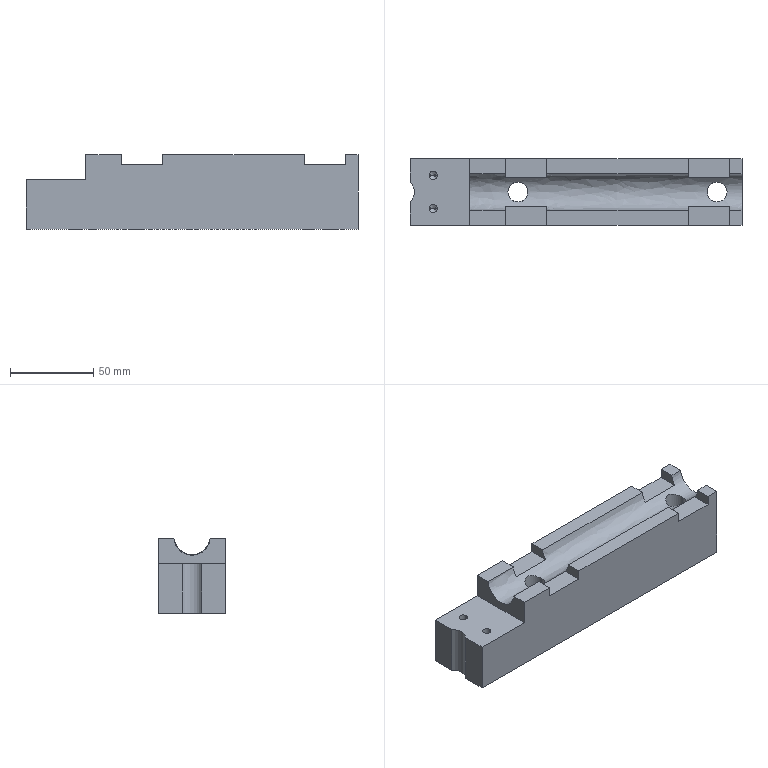NC program | NX | posted with a generic post
Lines 51 to 871 of 104568:
(ADAPTIVE_MILLING , TOOL : D10)
N100 T10 M6
N102 G54
N104 G17 G0 G90 X-107.551 Y-7.025 S9500 M3
N106 G43 Z30. H10
N108 Z-14.
N110 G94 G1 Z-15. F1000.
N112 X-105.318 Y-5.203 F3000.
N114 G3 X-104.997 Y-4.734 R1.064
N116 X-104.349 Y-0.599 R14.499
N118 X-104.258 Y2.898 R266.437
N120 X-104.741 Y3.891 R4.524
N122 G1 X-104.988 Y4.652
N124 G3 X-106.825 Y5.076 R1.102
N126 X-107.131 Y4.103 Z-14.947 R1.226
N128 G1 X-107.114 Y3.158 Z-14.9
N130 X-107.007 Y-2.847
N132 X-107. Y-3.483 Z-14.932
N134 X-106.969 Y-4.118 Z-14.964
N136 G3 X-106.617 Y-4.74 Z-15. R1.142
N138 X-104.842 Y-4.258 R1.102
N140 G2 X-104.254 Y-2.857 R24.923
N142 G3 X-103.658 Y2.081 R14.394
N144 X-104.235 Y2.995 R2.49
N146 G1 X-104.386 Y3.255
N148 G3 X-106.437 Y2.738 R1.101
N150 G1 X-106.619 Y-3.004
N152 G3 X-104.568 Y-3.591 R1.101
N154 X-103.136 Y1.38 R8.223
N156 X-103.8 Y2.451 R1.628
N158 G1 X-103.863 Y2.529
N160 G3 X-105.812 Y1.902 R1.101
N162 G1 X-106.065 Y-2.065
N164 G3 X-104.124 Y-2.842 R1.101
N166 X-102.749 Y1.145 R4.895
N168 G1 X-102.781 Y1.24
N170 X-102.821 Y1.331
N172 X-102.869 Y1.419
N174 G3 X-104.769 Y1.098 R1.102
N176 G1 X-105.607 Y-1.299
N178 G3 X-103.764 Y-2.412 R1.1
N180 X-102.442 Y-0.209 R3.842
N182 X-103.406 Y2.063 R2.803
N184 X-105.271 Y1.184 R1.101
N186 G1 X-105.076 Y-1.145
N188 G3 X-103.126 Y-1.747 R1.101
N190 X-102.442 Y-0.159 R2.495
N192 X-103.99 Y0.696 R1.012
N194 G1 X-104.991 Y0.067
N196 Z-12.
N198 G0 Z30.
N200 X-71.498 Y-27.794
N202 Z-13.849
N204 G1 Z-14.849 F1000.
N206 X-69.324 Y-25.783 F3000.
N208 G3 X-69. Y-25.042 R1.036
N210 X-71.916 Y-24.421 R8.181
N212 X-81.712 Y-24.21 R140.093
N214 G1 X-84.812 Y-24.207
N216 X-93.112 Y-24.205
N218 X-97.212
N220 X-97.312
N222 X-97.412 Y-24.203
N224 X-97.512 Y-24.198
N226 X-97.611 Y-24.192
N228 X-97.711 Y-24.183
N230 G2 X-102.043 Y-21.266 R6.063
N232 X-103.851 Y-15.497 R13.384
N234 X-104.115 Y-7.608 R54.303
N236 X-102.845 Y-3.623 R13.92
N238 G3 X-101.964 Y-0.266 R8.163
N240 X-102.667 Y1.898 R4.856
N242 G2 X-103.964 Y7.723 R17.087
N244 X-104.151 Y17.818 R129.978
N246 X-101.162 Y22.103 R6.099
N248 X-95.574 Y23.842 R13.466
N250 X-86.185 Y24.177 R90.73
N252 G3 X-70.586 Y24.227 R873.779
N254 X-69.295 Y24.665 R1.839
N256 X-69.022 Y25.112 R0.67
N258 X-69.69 Y26.058 R1.016
N260 G1 X-71.526 Y26.85 Z-14.749
N262 X-72.651 Y27.325
N264 X-72.919 Y27.362
N266 X-91.044
N268 G3 X-97.219 Y26.684 R28.808
N270 G1 X-98.437 Y26.413
N272 X-99.643 Y26.097
N274 G3 X-102.893 Y24.694 R14.612
N276 X-104.94 Y23.028 R10.254
N278 X-106.011 Y21.74 R8.094
N280 X-106.589 Y20.468 R5.588
N282 X-107.179 Y17.218 R15.413
N284 G1 X-107.231 Y16.391
N286 X-107.264 Y15.563
N288 X-107.597 Y-2.565
N290 G3 X-107.069 Y-13.778 R86.922
N292 G1 X-106.855 Y-15.681
N294 X-106.627 Y-17.583
N296 G3 X-105.191 Y-21.981 R14.894
N298 X-103.057 Y-24.999 R11.047
N300 G1 X-102.589 Y-25.467
N302 X-102.086 Y-25.898
N304 G3 X-100.53 Y-26.655 R4.838
N306 X-97.263 Y-27.212 R18.153
N308 G1 X-95.606 Y-27.319
N310 X-72.182 Y-28.224
N312 G3 X-71.516 Y-28.003 R1.032
N314 G1 X-70.11 Y-26.581 Z-14.849
N316 X-69.641 Y-26.109
N318 X-69.187 Y-25.623
N320 G3 X-69. Y-25.042 R1.045
N322 X-71.055 Y-24.079 R4.12
N324 X-77.516 Y-23.485 R33.131
N326 X-94.916 Y-23.403 R929.638
N328 G2 X-101.065 Y-19.485 R7.672
N330 X-102.98 Y-13.22 R15.729
N332 X-102.373 Y-5.318 R17.042
N334 G3 X-101.445 Y-1.132 R17.421
N336 X-101.971 Y1.806 R9.318
N338 G2 X-103.266 Y11.496 R40.447
N340 X-103.269 Y15.592 R31.14
N342 X-99.192 Y21.213 R7.783
N344 X-92.989 Y23.004 R16.193
N346 X-82.5 Y23.368 R104.354
N348 G3 X-71.702 Y23.449 R294.043
N350 X-69.296 Y24.284 R3.808
N352 X-69.022 Y25.021 R1.24
N354 X-69.691 Y25.969 R1.017
N356 G1 X-71.526 Y26.765 Z-14.749
N358 X-72.638 Y27.236
N360 X-72.919 Y27.271
N362 X-76.041 Y27.221
N364 X-79.162 Y27.12
N366 X-80.721 Y27.027
N368 X-82.278 Y26.917
N370 X-93.991 Y25.966
N372 G3 X-100.261 Y24.168 R16.575
N374 X-103.666 Y21.525 R13.673
N376 X-105.578 Y18.422 R7.953
N378 X-106.274 Y14.774 R14.488
N380 G1 X-106.563 Y9.89
N382 X-106.828 Y5.005
N384 G3 X-106.502 Y-8.29 R101.645
N386 G1 X-106.248 Y-11.134
N388 X-105.974 Y-13.977
N390 G3 X-104.543 Y-19.27 R19.249
N392 X-102.584 Y-22.402 R14.036
N394 G1 X-101.515 Y-23.672
N396 G3 X-98.586 Y-25.633 R8.09
N398 X-95.198 Y-26.339 R10.609
N400 G1 X-72.897 Y-27.292
N402 X-72.671 Y-27.272
N404 X-72.453 Y-27.208
N406 X-71.527 Y-26.802
N408 X-69.695 Y-26. Z-14.849
N410 G3 X-69. Y-25.042 R1.028
N412 X-70.551 Y-23.847 R2.838
N414 X-75.737 Y-22.862 R17.231
N416 X-87.532 Y-22.628 R195.199
N418 G2 X-93.331 Y-22.567 R112.761
N420 X-100.282 Y-17.783 R8.839
N422 X-101.664 Y-6.706 R16.242
N424 G3 X-100.864 Y-1.978 R34.974
N426 X-101.188 Y1.298 R14.457
N428 G2 X-102.425 Y13.113 R58.709
N430 X-97.864 Y20.191 R8.624
N432 X-91.193 Y22.152 R17.537
N434 X-81.706 Y22.549 R91.712
N436 G3 X-72.708 Y22.666 R202.321
N438 X-69.585 Y23.594 R6.019
N440 X-69.022 Y25.004 R1.448
N442 X-69.546 Y25.885 R1.011
N444 X-70.167 Y26.013 Z-14.817 R1.33
N446 G1 X-71.524 Y26.08 Z-14.749
N448 X-73.368 Y26.169
N450 X-77.742 Y26.174
N452 X-82.115 Y26.156
N454 G3 X-90.8 Y25.347 R61.155
N456 G1 X-94.989 Y24.639
N458 G3 X-99.124 Y22.965 R12.448
N460 G1 X-101.144 Y21.662
N462 G3 X-104.145 Y18.28 R9.835
N464 X-104.913 Y16.113 R8.633
N466 X-105.57 Y10.565 R27.18
N468 G1 X-105.757 Y-6.313
N470 G3 X-105.168 Y-12.5 R29.708
N472 X-104.358 Y-15.897 R32.087
N474 X-101.843 Y-21.056 R18.258
N476 X-98.772 Y-23.951 R11.298
N478 X-95.759 Y-25.144 R9.712
N480 X-92.685 Y-25.546 R16.686
N482 G1 X-73.263 Y-26.206
N484 X-71.527 Y-26.119
N486 X-69.811 Y-26.024 Z-14.835
N488 X-69.547 Y-25.933 Z-14.849
N490 G3 X-69. Y-25.042 R1.011
N492 X-70.13 Y-23.706 R2.222
N494 X-74.492 Y-22.349 R11.492
N496 X-83.774 Y-21.867 R75.922
N498 G2 X-91.572 Y-21.767 R185.382
N500 X-99.539 Y-16.175 R9.697
N502 X-100.826 Y-8.385 R14.411
N504 G3 X-100.227 Y-3.019 R231.829
N506 X-100.616 Y2.157 R25.935
N508 G2 X-101.499 Y11.306 R64.597
N510 X-96.577 Y19.253 R9.266
N512 X-89.524 Y21.322 R18.611
N514 X-78.537 Y21.747 R107.245
N516 G3 X-72.448 Y22.016 R46.627
N518 X-69.433 Y23.238 R5.711
N520 X-69.022 Y24.52 R1.468
N522 X-69.547 Y25.4 R1.011
N524 X-70.167 Y25.529 Z-14.817 R1.331
N526 G1 X-71.525 Y25.595 Z-14.749
N528 X-73.369 Y25.685
N530 X-77.534 Y25.673
N532 G3 X-82.716 Y25.272 R48.529
N534 G1 X-87.362 Y24.658
N536 X-92.005 Y24.022
N538 G3 X-98.894 Y21.283 R17.826
N540 X-101.285 Y19.489 R17.961
N542 X-103.973 Y14.822 R9.419
N544 X-104.324 Y12.737 R15.756
N546 X-104.616 Y9.008 R43.847
N548 X-104.645 Y1.146 R94.064
N550 G1 X-104.565 Y-0.349
N552 X-103.778 Y-12.828
N554 G3 X-102.349 Y-17.548 R10.682
N556 G1 X-100.862 Y-20.052
N558 G3 X-99.013 Y-21.984 R8.138
N560 X-94.577 Y-24.179 R12.587
N562 X-90.918 Y-24.867 R17.239
N564 G1 X-73.347 Y-26.206
N566 X-71.525 Y-26.121
N568 X-69.809 Y-26.023 Z-14.835
N570 X-69.544 Y-25.932 Z-14.849
N572 G3 X-69. Y-25.042 R1.011
N574 X-69.875 Y-23.538 R2.003
N576 X-73.699 Y-21.895 R9.077
N578 X-81.652 Y-21.144 R44.159
N580 G2 X-89.949 Y-20.975 R319.751
N582 X-99.206 Y-13.243 R10.229
N584 X-99.672 Y-6.99 R18.982
N586 G3 X-99.991 Y3.18 R42.362
N588 G2 X-100.553 Y9.752 R61.219
N590 X-95.226 Y18.421 R9.799
N592 X-87.966 Y20.499 R19.673
N594 X-77.78 Y20.945 R110.754
N596 G3 X-72.209 Y21.411 R29.071
N598 X-69.3 Y22.861 R5.501
N600 X-69.022 Y24.108 R1.707
N602 X-69.547 Y24.988 R1.011
N604 X-70.164 Y25.117 Z-14.817 R1.336
N606 G1 X-71.525 Y25.189 Z-14.749
N608 X-73.206 Y25.277
N610 X-73.369 Y25.272
N612 X-87.154 Y23.741
N614 G3 X-94.199 Y22.172 R33.647
N616 G1 X-95.251 Y21.815
N618 X-96.284 Y21.406
N620 G3 X-99.404 Y19.237 R10.854
N622 X-101.784 Y16.276 R13.511
N624 X-103.571 Y12.698 R44.582
N626 X-103.932 Y10.637 R5.47
N628 G1 X-103.599 Y-4.359
N630 G3 X-102.683 Y-11.765 R37.364
N632 G1 X-102.353 Y-13.227
N634 X-102.003 Y-14.685
N636 G3 X-101.245 Y-16.51 R9.099
N638 X-99.657 Y-19.043 R27.673
N640 X-97.843 Y-20.922 R11.68
N642 X-93.539 Y-23.281 R11.51
N644 X-91.118 Y-23.807 R15.167
N646 G1 X-73.256 Y-26.114
N648 X-71.525 Y-26.025
N650 X-69.808 Y-25.923 Z-14.835
N652 X-69.545 Y-25.832 Z-14.849
N654 G3 X-69. Y-24.942 R1.011
N656 X-69.906 Y-23.131 R2.265
N658 X-73.848 Y-21.275 R9.175
N660 X-81.485 Y-20.404 R38.939
N662 G2 X-88.68 Y-20.17 R205.805
N664 X-98.068 Y-12.319 R10.298
N666 X-98.679 Y-6.569 R22.003
N668 G3 X-99.267 Y3.706 R76.468
N670 G2 X-99.576 Y9.191 R34.592
N672 X-94.017 Y17.553 R10.207
N674 X-86.56 Y19.67 R20.395
N676 X-77.276 Y20.161 R125.201
N678 G3 X-71.837 Y20.871 R22.237
N680 X-69.213 Y22.432 R5.181
N682 X-69.023 Y23.581 R1.938
N684 X-69.6 Y24.488 R1.011
N686 X-70.505 Y24.479 Z-14.803 R1.154
N688 G1 X-71.525 Y24.161 Z-14.749
N690 X-72.452 Y23.87
N692 X-73.383 Y23.594
N694 X-75.013 Y23.543
N696 X-76.644 Y23.515
N698 G3 X-82.871 Y23.123 R76.701
N700 G1 X-85.461 Y22.853
N702 X-88.049 Y22.562
N704 G3 X-93.852 Y21.015 R25.49
N706 X-96.659 Y19.433 R15.104
N708 X-99.778 Y16.884 R27.516
N710 X-100.947 Y15.216 R6.294
N712 X-102.075 Y12.449 R24.754
N714 X-102.429 Y10.499 R8.848
N716 G1 X-102.575 Y8.186
N718 X-102.673 Y5.869
N720 G3 X-102.495 Y0.53 R51.707
N722 G1 X-101.629 Y-9.434
N724 G3 X-100.383 Y-14.868 R20.192
N726 X-98.162 Y-18.554 R13.351
N728 G1 X-97.017 Y-19.872
N730 G3 X-93.242 Y-22.175 R8.847
N732 X-88.993 Y-23.091 R20.48
N734 G1 X-73.403 Y-24.656
N736 X-71.527 Y-25.222
N738 X-70.153 Y-25.63 Z-14.821
N740 G3 X-69.599 Y-25.558 Z-14.849 R1.055
N742 X-69. Y-24.642 R1.01
N744 X-69.979 Y-22.646 R2.559
N746 X-74.061 Y-20.625 R9.568
N748 X-82.284 Y-19.627 R39.178
N750 G2 X-88.27 Y-19.274 R57.428
N752 X-96.862 Y-11.745 R10.375
N754 X-97.763 Y-5.526 R25.703
N756 G3 X-98.637 Y5.839 R344.55
N758 G2 X-97.195 Y12.674 R11.496
N760 X-90.93 Y17.565 R12.06
N762 X-83.096 Y19.049 R28.641
N764 G3 X-75.113 Y19.554 R220.804
N766 X-70.337 Y20.908 R12.291
N768 X-69.077 Y22.148 R2.767
N770 X-69.023 Y23.012 R4.341
N772 X-69.6 Y23.919 R1.011
N774 X-70.505 Y23.91 Z-14.803 R1.155
N776 G1 X-71.526 Y23.594 Z-14.749
N778 X-73.39 Y23.025
N780 X-76.017 Y22.929
N782 G3 X-80.986 Y22.517 R51.887
N784 G1 X-86.769 Y21.735
N786 G3 X-92.168 Y20.362 R29.535
N788 X-95.372 Y18.835 R21.075
N790 G1 X-96.799 Y17.979
N792 G3 X-98.255 Y16.556 R6.064
N794 X-100.231 Y13.382 R25.609
N796 X-101.584 Y9.382 R14.544
N798 X-101.716 Y7.399 R10.601
N800 G1 X-101.567 Y2.492
N802 X-101.394 Y-2.415
N804 G3 X-100.638 Y-8.782 R50.316
N806 G1 X-100.172 Y-11.235
N808 G3 X-97.267 Y-17.365 R15.298
N810 G1 X-96.558 Y-18.26
N812 X-95.838 Y-19.145
N814 G3 X-93.807 Y-20.672 R6.888
N816 X-91.362 Y-21.581 R12.433
N818 X-87.709 Y-22.363 R26.648
N820 G1 X-73.5 Y-24.342
N822 X-73.349 Y-24.375
N824 X-71.525 Y-24.926
N826 X-70.151 Y-25.33 Z-14.821
N828 G3 X-69.596 Y-25.256 Z-14.849 R1.054
N830 X-69. Y-24.342 R1.01
N832 X-70.022 Y-22.15 R2.81
N834 X-74.245 Y-19.971 R9.919
N836 X-82.255 Y-18.884 R37.047
N838 G2 X-87.823 Y-18.355 R34.863
N840 X-95.565 Y-11.515 R10.527
N842 X-96.885 Y-4.865 R25.565
N844 X-97.736 Y5.198 R295.524
N846 X-95.266 Y13.017 R11.166
N848 X-88.537 Y17.129 R13.662
N850 X-80.544 Y18.333 R37.68
N852 G3 X-73.688 Y19.065 R53.452
N854 X-69.682 Y20.777 R9.113
N856 X-69.023 Y22.422 R1.695
N858 X-69.599 Y23.328 R1.011
N860 X-70.5 Y23.323 Z-14.803 R1.157
N862 G1 X-71.526 Y23.012 Z-14.749
N864 X-73.357 Y22.457
N866 X-73.523 Y22.422
N868 X-84.686 Y21.027
N870 G3 X-91.319 Y19.355 R28.821
N872 X-94.793 Y17.433 R18.207
N874 X-97.379 Y15.413 R29.622
N876 X-99.15 Y12.943 R8.08
N878 X-99.893 Y10.958 R14.071
N880 X-100.635 Y7.311 R17.458
N882 X-100.819 Y1.284 R50.62
N884 X-100.502 Y-2.025 R31.857
N886 G1 X-99.946 Y-5.732
N888 X-99.367 Y-9.435
N890 G3 X-96.735 Y-15.692 R16.082
N892 X-95.247 Y-17.693 R25.842
N894 X-94.334 Y-18.535 R5.886
N896 X-91.25 Y-20.406 R15.587
N898 X-89.356 Y-21.004 R10.183
N900 X-79.553 Y-22.939 R395.254
N902 G1 X-73.392 Y-24.068
N904 X-71.522 Y-24.629
N906 X-70.149 Y-25.03 Z-14.821
N908 G3 X-69.593 Y-24.955 Z-14.849 R1.054
N910 X-69. Y-24.042 R1.01
N912 X-70.043 Y-21.65 R3.006
N914 X-74.406 Y-19.311 R10.29
N916 X-81.804 Y-18.169 R35.029
N918 G2 X-87.245 Y-17.442 R27.777
N920 X-94.402 Y-10.969 R10.885
N922 X-96.066 Y-3.886 R26.04
N924 X-96.815 Y4.677 R87.751
N926 X-90.536 Y15.039 R11.199
N928 X-82.975 Y17.181 R22.418
N930 G3 X-75.325 Y18.043 R321.614
N932 X-70.324 Y19.687 R13.269
N934 X-69.079 Y20.948 R2.96
N936 G1 X-69.052 Y21.044
N938 X-69.033 Y21.142
N940 G3 X-69.546 Y22.131 R1.01
N942 X-70.197 Y22.258 Z-14.816 R1.286
N944 G1 X-71.525 Y22.283 Z-14.749
N946 X-73.219 Y22.316
N948 X-73.379 Y22.307
N950 X-78.326 Y21.587
N952 G3 X-84.424 Y20.266 R62.869
N954 G1 X-86.644 Y19.667
N956 X-88.86 Y19.051
N958 G3 X-94.826 Y15.787 R17.967
N960 X-96.851 Y13.767 R19.041
N962 X-98.751 Y10.293 R10.937
N964 X-99.764 Y2.334 R18.501
N966 G1 X-99.441 Y-1.222
N968 X-99.096 Y-4.776
N970 G3 X-97.986 Y-9.99 R30.679
N972 G1 X-97.652 Y-11.076
N974 X-97.273 Y-12.146
N976 G3 X-95.956 Y-14.603 R13.344
N978 X-93.96 Y-17.113 R15.83
N980 X-91.994 Y-18.622 R9.756
N982 X-88.001 Y-20.293 R13.57
N984 G1 X-73.439 Y-23.658
N986 X-71.527 Y-24.229
N988 X-70.149 Y-24.63 Z-14.821
N990 G3 X-69.597 Y-24.557 Z-14.849 R1.055
N992 X-69. Y-23.642 R1.01
N994 X-70.048 Y-21.144 R3.159
N996 X-74.359 Y-18.708 R10.402
N998 X-81.733 Y-17.425 R35.048
N1000 G2 X-87.295 Y-16.281 R19.663
N1002 X-93.571 Y-9.756 R11.657
N1004 X-95.303 Y-2.686 R28.378
N1006 X-95.856 Y4.383 R42.163
N1008 X-89.464 Y14.191 R11.366
N1010 X-82.01 Y16.358 R23.26
N1012 G3 X-74.688 Y17.419 R130.567
N1014 X-69.985 Y19.29 R12.043
N1016 X-69.127 Y20.415 R1.86
N1018 X-69.024 Y21.919 R8.71
N1020 X-69.598 Y22.824 R1.011
N1022 X-70.497 Y22.822 Z-14.803 R1.158
N1024 G1 X-71.527 Y22.514 Z-14.749
N1026 X-73.524 Y21.919
N1028 X-84.438 Y19.19
N1030 G3 X-90.893 Y16.895 R35.793
N1032 X-94.35 Y14.689 R18.634
N1034 X-96.158 Y12.643 R11.095
N1036 X-97.987 Y9.39 R20.489
N1038 X-99.025 Y5.554 R13.162
N1040 X-99.051 Y3.338 R14.817
N1042 X-98.545 Y-1.626 R40.301
N1044 G1 X-98.097 Y-4.337
N1046 X-97.626 Y-7.044
N1048 G3 X-95.463 Y-12.943 R21.269
N1050 X-92.778 Y-16.327 R14.939
N1052 X-89.082 Y-18.774 R11.611
N1054 X-86.259 Y-19.755 R20.745
N1056 G1 X-73.471 Y-23.15
N1058 X-71.526 Y-23.73
N1060 X-70.148 Y-24.131 Z-14.821
N1062 G3 X-69.596 Y-24.056 Z-14.849 R1.055
N1064 X-69. Y-23.142 R1.01
N1066 X-70.04 Y-20.633 R3.27
N1068 X-74.582 Y-18.011 R10.7
N1070 X-80.553 Y-16.811 R32.516
N1072 G2 X-86.101 Y-15.579 R21.78
N1074 X-92.601 Y-8.981 R12.237
N1076 X-94.57 Y-1.357 R28.996
N1078 X-94.741 Y4.917 R21.079
N1080 X-88.458 Y13.322 R11.503
N1082 X-81.516 Y15.481 R23.464
N1084 G3 X-74.526 Y16.716 R121.257
N1086 X-69.96 Y18.665 R12.158
N1088 X-69.15 Y19.795 R1.885
N1090 G1 Y19.985
N1092 X-69.149 Y20.015
N1094 X-69.122 Y20.514
N1096 G3 X-69.623 Y21.437 R1.011
N1098 X-70.516 Y21.493 Z-14.803 R1.048
N1100 G1 X-71.54 Y21.167 Z-14.749
N1102 X-73.622 Y20.514
N1104 X-76.074 Y20.043
N1106 X-78.517 Y19.528
N1108 X-80.94 Y18.924
N1110 X-83.757 Y18.17
N1112 X-86.569 Y17.396
N1114 G3 X-91.447 Y15.331 R26.69
N1116 X-94.305 Y12.866 R10.092
N1118 X-96.965 Y8.383 R18.391
N1120 X-97.751 Y4.998 R12.013
N1122 X-97.921 Y1.622 R33.148
N1124 X-97.693 Y-1.212 R23.137
N1126 G1 X-97.415 Y-3.128
N1128 X-97.12 Y-5.042
N1130 G3 X-94.308 Y-12.114 R19.373
N1132 X-92.361 Y-14.823 R28.247
N1134 X-89.437 Y-17.213 R10.949
N1136 X-86.614 Y-18.492 R16.286
N1138 X-71.525 Y-23.33 R400.006
N1140 G1 X-70.148 Y-23.731 Z-14.821
N1142 G3 X-69.595 Y-23.656 Z-14.849 R1.055
N1144 X-69. Y-22.742 R1.01
N1146 X-70.085 Y-20.046 R3.447
N1148 X-74.79 Y-17.309 R11.147
N1150 X-80.647 Y-16.037 R39.14
N1152 G2 X-86.504 Y-14.119 R16.726
N1154 X-92.075 Y-7.263 R13.538
N1156 X-93.892 Y2.609 R26.202
N1158 X-87.766 Y12.295 R11.506
N1160 X-80.591 Y14.702 R24.163
N1162 G3 X-73.658 Y16.218 R71.536
N1164 X-69.763 Y18.191 R10.396
N1166 X-69.15 Y19.796 R1.7
N1168 X-69.694 Y20.686 R1.011
N1170 X-70.618 Y20.7 Z-14.801 R1.142
N1172 G1 X-71.621 Y20.4 Z-14.749
N1174 X-73.65 Y19.796
N1176 X-83.947 Y17.175
N1178 G3 X-89.648 Y14.731 R19.496
N1180 G1 X-90.669 Y14.019
N1182 X-91.616 Y13.307
N1184 X-92.553 Y12.584
N1186 G3 X-94.274 Y10.633 R9.506
N1188 X-96.461 Y6.171 R19.284
N1190 X-97.086 Y1.282 R12.39
N1192 X-95.698 Y-6.312 R34.347
N1194 X-93.131 Y-11.693 R21.216
N1196 G1 X-92.438 Y-12.731
N1198 X-91.709 Y-13.745
N1200 G3 X-90.845 Y-14.637 R5.947
N1202 G1 X-89.953 Y-15.374
N1204 X-89.032 Y-16.073
N1206 G3 X-86.124 Y-17.575 R14.009
N1208 G1 X-83.803 Y-18.495
N1210 X-81.464 Y-19.371
N1212 X-73.446 Y-22.259
N1214 X-71.524 Y-22.831
N1216 X-70.147 Y-23.231 Z-14.821
N1218 G3 X-69.594 Y-23.155 Z-14.849 R1.055
N1220 X-69. Y-22.242 R1.01
N1222 X-70.121 Y-19.455 R3.566
N1224 X-74.799 Y-16.667 R11.406
N1226 X-80.525 Y-15.262 R51.024
N1228 G2 X-87.325 Y-12.065 R14.769
N1230 X-91.726 Y-5.027 R15.77
N1232 X-92.796 Y2.446 R18.974
N1234 X-87.095 Y11.248 R11.396
N1236 X-80.097 Y13.856 R23.818
N1238 G3 X-73.225 Y15.626 R66.094
N1240 X-69.608 Y17.691 R9.466
N1242 X-69.15 Y18.5 R1.688
N1244 G1 Y19.2
N1246 G3 X-69.711 Y20.099 R1.011
N1248 X-70.621 Y20.103 Z-14.802 R1.151
N1250 G1 X-71.64 Y19.799 Z-14.749
N1252 X-75.645 Y18.626
N1254 X-79.66 Y17.483
N1256 G3 X-86.675 Y14.892 R50.238
N1258 G1 X-87.742 Y14.405
N1260 X-88.787 Y13.872
N1262 G3 X-91.772 Y11.487 R12.461
N1264 X-94.292 Y7.959 R14.287
N1266 X-95.572 Y3.826 R14.476
N1268 X-95.897 Y0.357 R18.253
N1270 X-95.669 Y-1.748 R15.107
N1272 X-94.785 Y-5.378 R22.524
N1274 G1 X-94.346 Y-6.679
N1276 X-93.858 Y-7.962
N1278 G3 X-91.561 Y-12.097 R22.611
N1280 X-89.417 Y-14.336 R10.613
N1282 X-85.708 Y-16.59 R15.813
N1284 G1 X-74.138 Y-21.48
N1286 X-73.405 Y-21.775
N1288 X-71.523 Y-22.333
N1290 X-70.146 Y-22.731 Z-14.821
N1292 G3 X-69.592 Y-22.655 Z-14.849 R1.055
N1294 X-69. Y-21.742 R1.01
N1296 X-70.491 Y-18.516 R4.187
N1298 X-75.734 Y-15.707 R13.214
N1300 G2 X-81.324 Y-14.166 R313.622
N1302 X-90.211 Y-5.944 R14.341
N1304 X-91.664 Y1.936 R15.949
N1306 X-86.27 Y10.291 R11.286
N1308 X-79.729 Y12.98 R23.393
N1310 G3 X-73.019 Y14.959 R69.414
N1312 X-69.55 Y17.082 R9.393
N1314 X-69.15 Y17.878 R1.494
N1316 G1 Y18.578
N1318 G3 X-69.711 Y19.476 R1.011
N1320 X-70.621 Y19.481 Z-14.802 R1.151
N1322 G1 X-71.639 Y19.177 Z-14.749
N1324 X-73.65 Y18.578
N1326 X-76.911 Y17.493
N1328 X-80.166 Y16.39
N1330 G3 X-85.98 Y13.894 R55.116
N1332 X-89.549 Y11.574 R21.428
N1334 G1 X-90.901 Y10.469
N1336 G3 X-92.91 Y7.951 R10.462
N1338 X-94.281 Y4.492 R12.102
N1340 G1 X-94.789 Y2.142
N1342 G3 X-94.82 Y-1.024 R10.303
N1344 X-93.94 Y-4.653 R21.171
N1346 G1 X-93.538 Y-5.834
N1348 X-93.089 Y-6.998
N1350 G3 X-91.417 Y-9.974 R17.92
N1352 X-89.387 Y-12.62 R28.362
N1354 X-86.94 Y-14.638 R11.286
N1356 X-81.98 Y-17.228 R35.867
N1358 G1 X-73.522 Y-20.801
N1360 X-71.539 Y-21.481
N1362 X-70.896 Y-21.707 Z-14.783
N1364 X-70.246 Y-21.912 Z-14.817
N1366 G3 X-69.627 Y-21.82 Z-14.849 R1.043
N1368 X-69.087 Y-20.776 R1.007
N1370 X-70.486 Y-17.954 R4.097
N1372 X-75.209 Y-15.22 R12.743
N1374 G2 X-80.632 Y-13.47 R292.103
N1376 X-90.529 Y0.184 R15.073
N1378 X-85.78 Y9.093 R10.904
N1380 X-79.474 Y12.063 R22.054
N1382 G3 X-73.022 Y14.201 R86.179
N1384 X-69.511 Y16.442 R9.511
N1386 X-69.15 Y17.169 R1.541
N1388 G1 Y17.969
N1390 G3 X-69.71 Y18.867 R1.011
N1392 X-70.619 Y18.873 Z-14.802 R1.151
N1394 G1 X-71.639 Y18.571 Z-14.749
N1396 X-73.65 Y17.969
N1398 X-84.568 Y13.31
N1400 G3 X-89.581 Y9.805 R14.965
N1402 X-92.158 Y6.353 R15.083
N1404 X-93.65 Y0.494 R12.419
N1406 G1 X-93.637 Y-1.278
N1408 G3 X-92.963 Y-4.43 R10.899
N1410 G1 X-92.481 Y-5.582
N1412 X-91.945 Y-6.711
N1414 G3 X-86.324 Y-13.8 R19.88
N1416 X-81.747 Y-16.576 R24.465
N1418 G1 X-73.631 Y-20.345
N1420 X-71.607 Y-20.986
N1422 X-70.945 Y-21.196 Z-14.784
N1424 X-70.279 Y-21.389 Z-14.818
N1426 G3 X-69.684 Y-21.295 Z-14.849 R1.046
N1428 X-69.131 Y-20.345 R1.01
N1430 X-70.344 Y-17.522 R3.87
N1432 X-74.882 Y-14.676 R12.428
N1434 G2 X-80.403 Y-12.599 R122.149
N1436 X-88.988 Y-2.551 R14.788
N1438 X-85.376 Y7.75 R10.366
N1440 X-78.993 Y11.211 R20.638
N1442 G3 X-72.72 Y13.56 R86.209
N1444 X-69.453 Y15.812 R9.199
N1446 X-69.15 Y16.464 R1.627
N1448 G1 Y17.264
N1450 G3 X-69.709 Y18.161 R1.011
N1452 X-70.618 Y18.169 Z-14.802 R1.151
N1454 G1 X-71.638 Y17.869 Z-14.749
N1456 X-73.504 Y17.32
N1458 X-73.65 Y17.264
N1460 X-82.686 Y12.978
N1462 G3 X-86.897 Y10.347 R21.831
N1464 G1 X-88.253 Y9.248
N1466 G3 X-90.28 Y6.744 R10.607
N1468 G1 X-90.583 Y6.199
N1470 X-90.866 Y5.645
N1472 X-91.603 Y4.06
N1474 G3 X-92.338 Y-0.314 R9.757
N1476 X-91.558 Y-4.581 R15.262
N1478 G1 X-91.181 Y-5.678
N1480 X-90.76 Y-6.759
N1482 G3 X-88.994 Y-9.628 R13.162
N1484 X-83.962 Y-13.996 R17.674
N1486 G1 X-73.544 Y-19.938
N1488 X-71.638 Y-20.496
N1490 X-70.962 Y-20.694 Z-14.784
N1492 X-70.283 Y-20.877 Z-14.819
N1494 G3 X-69.707 Y-20.782 Z-14.849 R1.049
N1496 X-69.15 Y-19.885 R1.011
N1498 X-70.224 Y-17.072 R3.742
N1500 X-74.67 Y-14.085 R12.376
N1502 G2 X-80.084 Y-11.746 R82.011
N1504 X-87.093 Y-4.485 R14.761
N1506 X-84.706 Y6.525 R9.83
N1508 X-78.534 Y10.339 R19.273
N1510 G3 X-72.544 Y12.858 R102.424
N1512 X-69.417 Y15.138 R9.174
N1514 X-69.15 Y15.782 R1.543
N1516 G1 Y16.482
N1518 G3 X-69.708 Y17.379 R1.011
N1520 X-70.617 Y17.387 Z-14.802 R1.151
N1522 G1 X-71.637 Y17.088 Z-14.749
N1524 X-73.568 Y16.518
N1526 X-82.035 Y12.289
N1528 G3 X-86.939 Y8.586 R16.983
N1530 G1 X-87.72 Y7.734
N1532 X-88.462 Y6.847
N1534 G3 X-90.765 Y0.985 R12.029
N1536 G1 X-90.906 Y-0.255
N1538 X-90.998 Y-1.5
N1540 G3 X-90.858 Y-2.728 R4.429
N1542 G1 X-90.537 Y-3.933
N1544 X-90.164 Y-5.122
N1546 G3 X-86.873 Y-10.342 R14.851
N1548 X-84.744 Y-12.373 R23.297
N1550 X-81.511 Y-14.411 R16.37
N1552 G1 X-73.416 Y-18.264
N1554 X-71.634 Y-19.547
N1556 X-70.609 Y-20.274 Z-14.812
N1558 G3 X-69.887 Y-20.35 Z-14.849 R1.03
N1560 X-69.15 Y-19.385 R1.007
N1562 X-70.294 Y-16.395 R3.899
N1564 X-74.446 Y-13.491 R12.95
N1566 G2 X-79.998 Y-10.739 R60.359
N1568 X-85.517 Y-4.965 R14.07
N1570 X-83.938 Y5.279 R9.287
N1572 X-78.294 Y9.338 R17.499
N1574 G3 X-72.416 Y12.111 R173.246
N1576 X-69.415 Y14.399 R9.498
N1578 X-69.15 Y15.041 R1.56
N1580 G1 Y15.841
N1582 G3 X-69.705 Y16.737 R1.011
N1584 X-70.612 Y16.749 Z-14.802 R1.153
N1586 G1 X-71.637 Y16.456 Z-14.749
N1588 X-73.529 Y15.905
N1590 X-73.65 Y15.841
N1592 X-81.626 Y10.926
N1594 G3 X-85.135 Y8.483 R37.614
N1596 X-88.966 Y2.85 R11.958
N1598 G1 X-89.463 Y1.213
N1600 G3 X-89.541 Y-2.604 R8.805
N1602 X-83.631 Y-11.919 R14.67
N1604 X-81.106 Y-13.513 R22.892
N1606 G1 X-77.242 Y-15.591
N1608 X-73.388 Y-17.689
N1610 X-71.635 Y-18.95
N1612 X-70.607 Y-19.675 Z-14.812
N1614 G3 X-69.886 Y-19.75 Z-14.849 R1.03
N1616 X-69.15 Y-18.785 R1.007
N1618 X-70.291 Y-15.79 R3.976
N1620 X-74.3 Y-12.85 R13.708
N1622 G2 X-79.948 Y-9.646 R47.465
N1624 X-84.233 Y-4.608 R12.025
N1626 X-82.811 Y4.332 R8.888
N1628 X-77.367 Y8.654 R17.109
N1630 G3 X-71.73 Y11.679 R111.53
N1632 X-69.277 Y13.848 R7.703
N1634 X-69.15 Y15.084 R2.757
N1636 X-69.705 Y15.98 R1.011
N1638 X-70.612 Y15.992 Z-14.802 R1.153
N1640 G1 X-71.636 Y15.698 Z-14.749
N1642 X-73.534 Y15.144
N1644 X-76.095 Y13.622
N1646 X-78.641 Y12.075
N1648 G3 X-83.718 Y7.846 R27.1
N1650 G1 X-84.717 Y6.786
N1652 X-85.7 Y5.711
N1654 G3 X-86.721 Y3.944 R6.427
N1656 X-87.663 Y0.974 R29.362
N1658 X-88.014 Y-1.692 R11.7
N1660 X-87.801 Y-3.324 R7.45
N1662 X-86.231 Y-7.359 R13.717
N1664 X-83.53 Y-10.666 R15.379
N1666 X-79.671 Y-13.554 R18.694
N1668 G1 X-73.403 Y-17.08
N1670 X-71.634 Y-18.351
N1672 X-70.607 Y-19.075 Z-14.812
N1674 G3 X-69.885 Y-19.15 Z-14.849 R1.03
N1676 X-69.15 Y-18.185 R1.007
N1678 X-70.279 Y-15.182 R4.028
N1680 X-74.22 Y-12.145 R14.877
N1682 G2 X-79.602 Y-8.697 R39.316
N1684 X-83.067 Y-3.459 R9.593
N1686 X-81.078 Y4.111 R8.982
N1688 X-76.076 Y8.207 R18.395
N1690 G3 X-71.05 Y11.293 R65.411
N1692 X-69.24 Y13.131 R6.352
N1694 X-69.15 Y14.295 R3.285
N1696 X-69.7 Y15.188 R1.011
N1698 X-70.6 Y15.209 Z-14.803 R1.157
N1700 G1 X-71.636 Y14.927 Z-14.749
N1702 X-73.417 Y14.434
N1704 X-73.65 Y14.295
N1706 X-80.977 Y8.447
N1708 G3 X-84.468 Y4.584 R16.814
N1710 X-85.806 Y2.24 R18.727
N1712 X-86.407 Y-0.885 R7.217
N1714 G1 X-86.331 Y-2.663
N1716 G3 X-83.676 Y-8.912 R11.155
N1718 X-80.059 Y-12.16 R15.985
N1720 G1 X-73.459 Y-16.446
N1722 X-71.636 Y-17.751
N1724 X-70.606 Y-18.476 Z-14.812
N1726 G3 X-69.886 Y-18.55 Z-14.849 R1.03
N1728 X-69.15 Y-17.585 R1.007
N1730 X-70.259 Y-14.572 R4.102
N1732 X-74.286 Y-11.317 R16.838
N1734 G2 X-78.825 Y-8.051 R30.45